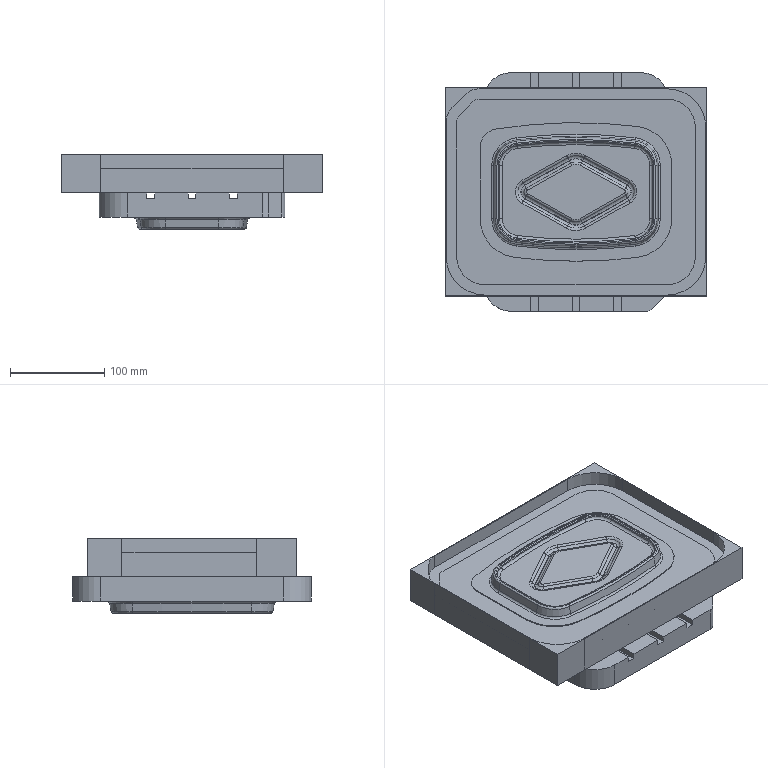NC program | NX | posted with a generic post | part box 278.144 x 254.144 x 79 mm
Lines 4246 to 4920 of 124328:
(CAVITY_MILL_1_COPY , TOOL : D4)
N8490 M6
N8492 G53
N8494 G17 G0 G90 X71.275 Y-37.886 S7000 M3 M8
N8496 G43 Z100.5 H0
N8498 Z37.033
N8500 G94 G1 Z36.033 F4500.
N8502 X72.559 Y-38.883
N8504 G3 X73.682 Y-38.742 R0.8
N8506 G1 X73.795 Y-38.595
N8508 X73.823 Y-38.558
N8510 G3 X74.043 Y-38.269 R17.033
N8512 G2 X76.737 Y-37.786 R2.
N8514 X66.818 Y-46.033 R18.553
N8516 X64.72 Y-46.628 R23.515
N8518 X65.993 Y-44.199 R2.
N8520 G3 X73.309 Y-39.205 R16.805
N8522 G1 X73.341 Y-39.166
N8524 G3 X73.682 Y-38.742 R16.926
N8526 X73.541 Y-37.619 R0.8
N8528 G1 X72.275 Y-36.637
N8530 Z37.033
N8532 G0 Z43.5
N8534 X60.026 Y-40.649
N8536 Z35.13
N8538 G1 Z34.13
N8540 X60.404 Y-42.151
N8542 G3 X61.375 Y-42.731 R0.8
N8544 G1 X61.449 Y-42.712
N8546 G2 X63.94 Y-44.23 R2.
N8548 X63.391 Y-44.336 R16.076
N8550 G1 X62.289 Y-44.523
N8552 G3 X61.928 Y-44.677 R0.84
N8554 G2 X59.759 Y-44.937 R511.246
N8556 X61.301 Y-42.749 R2.
N8558 G1 X61.375 Y-42.731
N8560 G3 X61.956 Y-41.76 R0.8
N8562 G1 X61.577 Y-40.258
N8564 Z35.13
N8566 G0 Z39.033
N8568 X73.119 Y-30.779
N8570 Z35.13
N8572 G1 Z34.13
N8574 X75.709 Y-31.085
N8576 G3 X76.597 Y-30.385 R0.8
N8578 X76.696 Y-29.123 R16.076
N8580 G2 X76.842 Y-28.323 R2.892
N8582 G1 Y-26.204
N8584 G3 X76.042 Y-25.404 R0.8
N8586 G1 X73.448
N8588 Z35.13
N8590 G0 Z41.65
N8592 X-2.129 Y103.007
N8594 Z27.506
N8596 G1 Z26.506
N8598 Y106.722
N8600 G3 X-2.929 Y107.522 R0.8
N8602 G1 X97.072
N8604 G2 X135.922 Y68.672 R38.85
N8606 G1 Y-68.672
N8608 G2 X97.072 Y-107.522 R38.85
N8610 G1 X-97.072
N8612 G2 X-135.922 Y-68.672 R38.85
N8614 G1 Y74.53
N8616 G2 X-130.401 Y87.859 R18.85
N8618 G1 X-116.259 Y102.001
N8620 G2 X-102.93 Y107.522 R18.85
N8622 G1 X-2.929
N8624 Y105.722
N8626 X97.072
N8628 G2 X134.122 Y68.672 R37.05
N8630 G1 Y-68.672
N8632 G2 X97.072 Y-105.722 R37.05
N8634 G1 X-97.072
N8636 G2 X-134.122 Y-68.672 R37.05
N8638 G1 Y74.53
N8640 G2 X-129.128 Y86.586 R17.05
N8642 G1 X-114.986 Y100.728
N8644 G2 X-102.93 Y105.722 R17.05
N8646 G1 X-2.929
N8648 G3 X-2.129 Y106.522 R0.8
N8650 G1 Y103.007
N8652 Z27.506
N8654 G0 Z29.756
N8656 Y103.006 Z27.256
N8658 G1 Z26.256
N8660 Y106.722
N8662 G3 X-2.929 Y107.522 R0.8
N8664 G1 X97.072
N8666 G2 X135.922 Y68.672 R38.85
N8668 G1 Y-68.672
N8670 G2 X97.072 Y-107.522 R38.85
N8672 G1 X-97.072
N8674 G2 X-135.922 Y-68.672 R38.85
N8676 G1 Y74.53
N8678 G2 X-130.401 Y87.859 R18.85
N8680 G1 X-116.259 Y102.001
N8682 G2 X-102.93 Y107.522 R18.85
N8684 G1 X-2.929
N8686 Y105.722
N8688 X97.072
N8690 G2 X134.122 Y68.672 R37.05
N8692 G1 Y-68.672
N8694 G2 X97.072 Y-105.722 R37.05
N8696 G1 X-97.072
N8698 G2 X-134.122 Y-68.672 R37.05
N8700 G1 Y74.53
N8702 G2 X-129.128 Y86.586 R17.05
N8704 G1 X-114.986 Y100.728
N8706 G2 X-102.93 Y105.722 R17.05
N8708 G1 X-2.929
N8710 G3 X-2.129 Y106.522 R0.8
N8712 G1 Y103.006
N8714 Z27.256
N8716 G0 Z29.506
N8718 X-26.78 Y107.522
N8720 Z27.256
N8722 G1 X-2.929 Z26.006
N8724 X97.072
N8726 G2 X135.922 Y68.672 R38.85
N8728 G1 Y-68.672
N8730 G2 X97.072 Y-107.522 R38.85
N8732 G1 X-97.072
N8734 G2 X-135.922 Y-68.672 R38.85
N8736 G1 Y74.53
N8738 G2 X-130.401 Y87.859 R18.85
N8740 G1 X-116.259 Y102.001
N8742 G2 X-102.93 Y107.522 R18.85
N8744 G1 X-2.929
N8746 Y105.722
N8748 X97.072
N8750 G2 X134.122 Y68.672 R37.05
N8752 G1 Y-68.672
N8754 G2 X97.072 Y-105.722 R37.05
N8756 G1 X-97.072
N8758 G2 X-134.122 Y-68.672 R37.05
N8760 G1 Y74.53
N8762 G2 X-129.128 Y86.586 R17.05
N8764 G1 X-114.986 Y100.728
N8766 G2 X-102.93 Y105.722 R17.05
N8768 G1 X-2.929
N8770 G3 X-2.129 Y106.522 R0.8
N8772 G1 Y102.782
N8774 Z27.006
N8776 G0 Z29.256
N8778 X-26.78 Y107.522
N8780 Z27.006
N8782 G1 X-2.929 Z25.756
N8784 X97.072
N8786 G2 X135.922 Y68.672 R38.85
N8788 G1 Y-68.672
N8790 G2 X97.072 Y-107.522 R38.85
N8792 G1 X-97.072
N8794 G2 X-135.922 Y-68.672 R38.85
N8796 G1 Y74.53
N8798 G2 X-130.401 Y87.859 R18.85
N8800 G1 X-116.259 Y102.001
N8802 G2 X-102.93 Y107.522 R18.85
N8804 G1 X-2.929
N8806 Y105.722
N8808 X97.072
N8810 G2 X134.122 Y68.672 R37.05
N8812 G1 Y-68.672
N8814 G2 X97.072 Y-105.722 R37.05
N8816 G1 X-97.072
N8818 G2 X-134.122 Y-68.672 R37.05
N8820 G1 Y74.53
N8822 G2 X-129.128 Y86.586 R17.05
N8824 G1 X-114.986 Y100.728
N8826 G2 X-102.93 Y105.722 R17.05
N8828 G1 X-2.929
N8830 G3 X-2.129 Y106.522 R0.8
N8832 G1 Y102.382
N8834 Z26.756
N8836 G0 Z41.65
N8838 X11.778 Y34.008
N8840 Z35.13
N8842 G1 X32.543 Y22.591 Z33.889
N8844 X55.835 Y9.784
N8846 G2 X55.951 Y-8.882 R10.688
N8848 G1 X8.639 Y-35.664
N8850 G2 X-8.677 Y-35.713 R17.663
N8852 G1 X-55.899 Y-9.33
N8854 G2 X-55.888 Y9.336 R10.688
N8856 G1 X-8.535 Y35.722
N8858 G2 X8.573 Y35.771 R17.663
N8860 G1 X32.543 Y22.591
N8862 X31.194 Y20.137
N8864 X54.486 Y7.33
N8866 G2 X54.572 Y-6.446 R7.888
N8868 G1 X7.26 Y-33.227
N8870 G2 X-7.312 Y-33.268 R14.863
N8872 G1 X-54.533 Y-6.886
N8874 G2 X-54.525 Y6.89 R7.888
N8876 G1 X-7.172 Y33.276
N8878 G2 X7.224 Y33.317 R14.863
N8880 G1 X31.194 Y20.137
N8882 X30.327 Y18.56
N8884 X53.619 Y5.753
N8886 G2 X53.685 Y-4.879 R6.088
N8888 G1 X6.373 Y-31.661
N8890 G2 X-6.434 Y-31.697 R13.063
N8892 G1 X-53.655 Y-5.315
N8894 G2 X-53.649 Y5.318 R6.088
N8896 G1 X-6.296 Y31.704
N8898 G2 X6.356 Y31.74 R13.063
N8900 G1 X30.327 Y18.56
N8902 G3 X31.413 Y18.875 R0.8
N8904 G1 Z34.889
N8906 G0 Z37.13
N8908 X7.26 Y-33.227
N8910 Z34.889
N8912 G1 Z33.889
N8914 X5.963 Y-30.937
N8916 G2 X-6.028 Y-30.971 R12.232
N8918 G1 X-53.25 Y-4.589
N8920 G2 X-53.245 Y4.592 R5.256
N8922 G1 X-5.892 Y30.978
N8924 G2 X5.956 Y31.011 R12.232
N8926 G1 X53.219 Y5.024
N8928 G2 X53.275 Y-4.156 R5.256
N8930 G1 X5.963 Y-30.937
N8932 G3 X5.661 Y-32.028 R0.8
N8934 G1 Z34.889
N8936 G0 Z37.13
N8938 X11.211 Y33.779
N8940 Z34.889
N8942 G1 X31.975 Y22.362 Z33.647
N8944 X55.607 Y9.368
N8946 G2 X55.717 Y-8.47 R10.213
N8948 G1 X8.405 Y-35.251
N8950 G2 X-8.446 Y-35.298 R17.189
N8952 G1 X-55.667 Y-8.916
N8954 G2 X-55.657 Y8.922 R10.213
N8956 G1 X-8.304 Y35.308
N8958 G2 X8.344 Y35.355 R17.189
N8960 G1 X31.975 Y22.362
N8962 X30.626 Y19.908
N8964 X54.258 Y6.915
N8966 G2 X54.338 Y-6.033 R7.413
N8968 G1 X7.026 Y-32.815
N8970 G2 X-7.08 Y-32.854 R14.389
N8972 G1 X-54.302 Y-6.472
N8974 G2 X-54.294 Y6.476 R7.413
N8976 G1 X-6.941 Y32.862
N8978 G2 X6.995 Y32.901 R14.389
N8980 G1 X30.626 Y19.908
N8982 X29.816 Y18.434
N8984 X53.447 Y5.44
N8986 G2 X53.509 Y-4.569 R5.731
N8988 G1 X6.197 Y-31.35
N8990 G2 X-6.26 Y-31.385 R12.706
N8992 G1 X-53.481 Y-5.003
N8994 G2 X-53.475 Y5.006 R5.731
N8996 G1 X-6.122 Y31.392
N8998 G2 X6.184 Y31.427 R12.706
N9000 G1 X29.816 Y18.434
N9002 G3 X30.902 Y18.749 R0.8
N9004 G1 Z34.647
N9006 G0 Z36.889
N9008 X11.047 Y33.481
N9010 Z34.647
N9012 G1 X31.812 Y22.064 Z33.405
N9014 X55.443 Y9.07
N9016 G2 X55.55 Y-8.174 R9.873
N9018 G1 X8.238 Y-34.955
N9020 G2 X-8.28 Y-35.002 R16.849
N9022 G1 X-55.502 Y-8.619
N9024 G2 X-55.492 Y8.625 R9.873
N9026 G1 X-8.139 Y35.011
N9028 G2 X8.18 Y35.057 R16.849
N9030 G1 X31.812 Y22.064
N9032 X30.463 Y19.61
N9034 X54.094 Y6.617
N9036 G2 X54.17 Y-5.737 R7.073
N9038 G1 X6.858 Y-32.519
N9040 G2 X-6.914 Y-32.557 R14.049
N9042 G1 X-54.136 Y-6.175
N9044 G2 X-54.129 Y6.179 R7.073
N9046 G1 X-6.776 Y32.565
N9048 G2 X6.831 Y32.603 R14.049
N9050 G1 X30.463 Y19.61
N9052 X29.98 Y18.731
N9054 X53.611 Y5.738
N9056 G2 X53.677 Y-4.864 R6.071
N9058 G1 X6.364 Y-31.646
N9060 G2 X-6.425 Y-31.682 R13.046
N9062 G1 X-53.647 Y-5.3
N9064 G2 X-53.641 Y5.303 R6.071
N9066 G1 X-6.288 Y31.689
N9068 G2 X6.348 Y31.725 R13.046
N9070 G1 X29.98 Y18.731
N9072 G3 X31.066 Y19.047 R0.8
N9074 G1 Z34.405
N9076 G0 Z36.647
N9078 X11.417 Y32.974
N9080 Z34.405
N9082 G1 X32.182 Y21.557 Z33.163
N9084 X55.315 Y8.837
N9086 G2 X55.419 Y-7.943 R9.608
N9088 G1 X8.107 Y-34.724
N9090 G2 X-8.15 Y-34.77 R16.583
N9092 G1 X-55.372 Y-8.387
N9094 G2 X-55.363 Y8.393 R9.608
N9096 G1 X-8.01 Y34.779
N9098 G2 X8.052 Y34.824 R16.583
N9100 G1 X32.182 Y21.557
N9102 X31.315 Y19.979
N9104 X54.448 Y7.26
N9106 G2 X54.532 Y-6.376 R7.808
N9108 G1 X7.22 Y-33.158
N9110 G2 X-7.273 Y-33.198 R14.783
N9112 G1 X-54.494 Y-6.816
N9114 G2 X-54.486 Y6.82 R7.808
N9116 G1 X-7.133 Y33.206
N9118 G2 X7.185 Y33.247 R14.783
N9120 G1 X31.315 Y19.979
N9122 G3 X32.401 Y20.295 R0.8
N9124 G1 Z34.163
N9126 G0 Z36.405
N9128 X8.107 Y-34.724
N9130 Z34.163
N9132 G1 Z33.163
N9134 X6.495 Y-31.877
N9136 G2 X-6.555 Y-31.914 R13.312
N9138 G1 X-53.777 Y-5.532
N9140 G2 X-53.77 Y5.535 R6.336
N9142 G1 X-6.417 Y31.921
N9144 G2 X6.476 Y31.958 R13.312
N9146 G1 X53.739 Y5.971
N9148 G2 X53.807 Y-5.096 R6.336
N9150 G1 X6.495 Y-31.877
N9152 G3 X6.193 Y-32.968 R0.8
N9154 G1 Z34.163
N9156 G0 Z36.405
N9158 X11.314 Y32.786
N9160 Z34.163
N9162 G1 X32.078 Y21.368 Z32.921
N9164 X55.211 Y8.649
N9166 G2 X55.313 Y-7.755 R9.393
N9168 G1 X8.001 Y-34.537
N9170 G2 X-8.046 Y-34.582 R16.368
N9172 G1 X-55.267 Y-8.2
N9174 G2 X-55.258 Y8.205 R9.393
N9176 G1 X-7.905 Y34.591
N9178 G2 X7.949 Y34.636 R16.368
N9180 G1 X32.078 Y21.368
N9182 X31.211 Y19.791
N9184 X54.344 Y7.072
N9186 G2 X54.426 Y-6.189 R7.593
N9188 G1 X7.114 Y-32.971
N9190 G2 X-7.168 Y-33.011 R14.568
N9192 G1 X-54.389 Y-6.628
N9194 G2 X-54.382 Y6.632 R7.593
N9196 G1 X-7.029 Y33.019
N9198 G2 X7.081 Y33.058 R14.568
N9200 G1 X31.211 Y19.791
N9202 G3 X32.298 Y20.107 R0.8
N9204 G1 Z33.921
N9206 G0 Z37.13
N9208 X8.001 Y-34.537
N9210 Z33.921
N9212 G1 Z32.921
N9214 X6.601 Y-32.065
N9216 G2 X-6.66 Y-32.102 R13.527
N9218 G1 X-53.881 Y-5.719
N9220 G2 X-53.875 Y5.723 R6.551
N9222 G1 X-6.522 Y32.109
N9224 G2 X6.58 Y32.146 R13.527
N9226 G1 X53.843 Y6.159
N9228 G2 X53.913 Y-5.283 R6.551
N9230 G1 X6.601 Y-32.065
N9232 G3 X6.299 Y-33.155 R0.8
N9234 G1 Z33.921
N9236 G0 Z37.13
N9238 X11.229 Y32.631
N9240 Z33.921
N9242 G1 X31.993 Y21.214 Z32.679
N9244 X55.126 Y8.494
N9246 G2 X55.226 Y-7.602 R9.216
N9248 G1 X7.914 Y-34.383
N9250 G2 X-7.96 Y-34.428 R16.192
N9252 G1 X-55.181 Y-8.046
N9254 G2 X-55.172 Y8.051 R9.216
N9256 G1 X-7.819 Y34.437
N9258 G2 X7.864 Y34.481 R16.192
N9260 G1 X31.993 Y21.214
N9262 X31.126 Y19.636
N9264 X54.259 Y6.917
N9266 G2 X54.339 Y-6.035 R7.416
N9268 G1 X7.027 Y-32.817
N9270 G2 X-7.082 Y-32.856 R14.392
N9272 G1 X-54.303 Y-6.474
N9274 G2 X-54.296 Y6.478 R7.416
N9276 G1 X-6.943 Y32.864
N9278 G2 X6.996 Y32.904 R14.392
N9280 G1 X31.126 Y19.636
N9282 G3 X32.213 Y19.952 R0.8
N9284 G1 Z33.679
N9286 G0 Z37.13
N9288 X7.914 Y-34.383
N9290 Z33.679
N9292 G1 Z32.679
N9294 X6.688 Y-32.218
N9296 G2 X-6.746 Y-32.256 R13.703
N9298 G1 X-53.967 Y-5.873
N9300 G2 X-53.961 Y5.877 R6.728
N9302 G1 X-6.608 Y32.263
N9304 G2 X6.665 Y32.301 R13.703
N9306 G1 X53.928 Y6.314
N9308 G2 X54. Y-5.436 R6.728
N9310 G1 X6.688 Y-32.218
N9312 G3 X6.386 Y-33.308 R0.8
N9314 G1 Z33.679
N9316 G0 Z37.13
N9318 X11.146 Y32.48
N9320 Z33.679
N9322 G1 X31.91 Y21.063 Z32.437
N9324 X55.043 Y8.343
N9326 G2 X55.141 Y-7.452 R9.044
N9328 G1 X7.829 Y-34.234
N9330 G2 X-7.875 Y-34.277 R16.019
N9332 G1 X-55.097 Y-7.895
N9334 G2 X-55.088 Y7.9 R9.044
N9336 G1 X-7.735 Y34.286
N9338 G2 X7.781 Y34.33 R16.019
N9340 G1 X31.91 Y21.063
N9342 X30.878 Y19.184
N9344 X54.011 Y6.465
N9346 G2 X54.085 Y-5.586 R6.9
N9348 G1 X6.773 Y-32.368
N9350 G2 X-6.83 Y-32.406 R13.876
N9352 G1 X-54.052 Y-6.024
N9354 G2 X-54.045 Y6.028 R6.9
N9356 G1 X-6.692 Y32.414
N9358 G2 X6.748 Y32.452 R13.876
N9360 G1 X30.878 Y19.184
N9362 G3 X31.964 Y19.5 R0.8
N9364 G1 Z33.437
N9366 G0 Z35.679
N9368 X11.047 Y32.301
N9370 Z33.437
N9372 G1 X31.812 Y20.884 Z32.195
N9374 X54.945 Y8.165
N9376 G2 X55.041 Y-7.274 R8.84
N9378 G1 X7.728 Y-34.056
N9380 G2 X-7.776 Y-34.099 R15.815
N9382 G1 X-54.997 Y-7.717
N9384 G2 X-54.989 Y7.722 R8.84
N9386 G1 X-7.636 Y34.108
N9388 G2 X7.682 Y34.151 R15.815
N9390 G1 X31.812 Y20.884
N9392 X30.976 Y19.363
N9394 X54.109 Y6.644
N9396 G2 X54.186 Y-5.764 R7.104
N9398 G1 X6.874 Y-32.546
N9400 G2 X-6.93 Y-32.584 R14.08
N9402 G1 X-54.151 Y-6.202
N9404 G2 X-54.144 Y6.206 R7.104
N9406 G1 X-6.791 Y32.592
N9408 G2 X6.846 Y32.631 R14.08
N9410 G1 X30.976 Y19.363
N9412 G3 X32.062 Y19.679 R0.8
N9414 G1 Z33.195
N9416 G0 Z35.437
N9418 X10.431 Y32.362
N9420 Z33.195
N9422 G1 X31.196 Y20.944 Z31.953
N9424 X54.828 Y7.951
N9426 G2 X54.921 Y-7.062 R8.596
N9428 G1 X7.608 Y-33.844
N9430 G2 X-7.657 Y-33.887 R15.572
N9432 G1 X-54.879 Y-7.504
N9434 G2 X-54.87 Y7.509 R8.596
N9436 G1 X-7.517 Y33.895
N9438 G2 X7.565 Y33.938 R15.572
N9440 G1 X31.196 Y20.944
N9442 X30.595 Y19.851
N9444 X54.226 Y6.857
N9446 G2 X54.306 Y-5.976 R7.348
N9448 G1 X6.994 Y-32.758
N9450 G2 X-7.048 Y-32.797 R14.323
N9452 G1 X-54.27 Y-6.415
N9454 G2 X-54.263 Y6.419 R7.348
N9456 G1 X-6.91 Y32.805
N9458 G2 X6.964 Y32.844 R14.323
N9460 G1 X30.595 Y19.851
N9462 G3 X31.681 Y20.166 R0.8
N9464 G1 Z32.953
N9466 G0 Z35.195
N9468 X10.289 Y32.102
N9470 Z32.953
N9472 G1 X31.053 Y20.685 Z31.712
N9474 X54.685 Y7.691
N9476 G2 X54.775 Y-6.804 R8.3
N9478 G1 X7.462 Y-33.586
N9480 G2 X-7.513 Y-33.628 R15.275
N9482 G1 X-54.734 Y-7.246
N9484 G2 X-54.726 Y7.25 R8.3
N9486 G1 X-7.373 Y33.636
N9488 G2 X7.422 Y33.678 R15.275
N9490 G1 X31.053 Y20.685
N9492 X30.738 Y20.11
N9494 X54.369 Y7.117
N9496 G2 X54.452 Y-6.234 R7.644
N9498 G1 X7.14 Y-33.016
N9500 G2 X-7.193 Y-33.056 R14.62
N9502 G1 X-54.414 Y-6.673
N9504 G2 X-54.407 Y6.678 R7.644
N9506 G1 X-7.054 Y33.064
N9508 G2 X7.106 Y33.104 R14.62
N9510 G1 X30.738 Y20.11
N9512 G3 X31.281 Y20.268 R0.4
N9514 G1 Z32.712
N9516 G0 Z41.65
N9518 X-108.649 Y8.666
N9520 Z27.506
N9522 G1 Z26.506
N9524 X-107.049
N9526 G3 X-106.249 Y9.466 R0.8
N9528 G1 Y47.133
N9530 G2 X-85.957 Y70.972 R24.149
N9532 G1 X-85.955
N9534 G2 X65.889 Y73.819 R540.653
N9536 X106.249 Y28.201 R45.961
N9538 G1 Y-28.201
N9540 G2 X65.889 Y-73.819 R45.961
N9542 X-65.889 Y-73.819 R540.653
N9544 X-106.249 Y-28.201 R45.961
N9546 G1 Y9.466
N9548 X-104.222
N9550 Y47.133
N9552 G2 X-85.616 Y68.974 R22.122
N9554 X65.642 Y71.807 R538.627
N9556 X104.222 Y28.201 R43.934
N9558 G1 Y-28.201
N9560 G2 X65.642 Y-71.807 R43.934
N9562 X-65.642 Y-71.807 R538.627
N9564 X-104.222 Y-28.201 R43.934
N9566 G1 Y9.466
N9568 G3 X-105.022 Y10.266 R0.8
N9570 G1 X-108.649
N9572 Z27.506
N9574 G0 Z29.756
N9576 X-108.726 Y8.666
N9578 Z27.256
N9580 G1 Z26.256
N9582 X-107.126
N9584 G3 X-106.326 Y9.466 R0.8
N9586 G1 Y46.996
N9588 X-106.325 Y47.066
N9590 Y47.133
N9592 G2 X-85.952 Y71.051 R24.226
N9594 X65.856 Y73.9 R540.73
N9596 G1 X65.859
N9598 X65.863 Y73.899
N9600 G2 X106.325 Y28.421 R46.037
N9602 G1 X106.324 Y28.3
N9604 G3 X106.324 Y28.093 R3.884
N9606 G1 X106.326 Y27.981
N9608 Y-27.981
N9610 X106.324 Y-28.092
N9612 G3 X106.324 Y-28.3 R3.884
N9614 G1 X106.325 Y-28.421
N9616 G2 X65.904 Y-73.894 R46.037
N9618 X-65.856 Y-73.9 R540.73
N9620 G1 X-65.86
N9622 G2 X-106.325 Y-28.421 R46.037
N9624 G1 X-106.324 Y-28.3
N9626 G3 X-106.324 Y-28.093 R3.885
N9628 G1 X-106.326 Y-27.981
N9630 Y9.466
N9632 X-104.222
N9634 Y47.133
N9636 G2 X-85.616 Y68.974 R22.122
N9638 X65.642 Y71.807 R538.627
N9640 X104.222 Y28.201 R43.934
N9642 G1 Y-28.201
N9644 G2 X65.642 Y-71.807 R43.934
N9646 X-65.642 Y-71.807 R538.627
N9648 X-104.222 Y-28.201 R43.934
N9650 G1 Y9.466
N9652 G3 X-105.022 Y10.266 R0.8
N9654 G1 X-108.726
N9656 Z27.256
N9658 G0 Z29.506
N9660 X-108.958 Y8.666
N9662 Z27.006
N9664 G1 Z26.006
N9666 X-107.358
N9668 G3 X-106.558 Y9.466 R0.8
N9670 G1 Y47.017
N9672 X-106.557 Y47.078
N9674 Y47.133
N9676 G2 X-85.988 Y71.28 R24.457
N9678 G1 X-85.987
N9680 G2 X65.885 Y74.13 R540.962
N9682 G1 X65.883
N9684 X65.888
N9686 G2 X106.558 Y28.163 R46.269
N9688 G1 Y28.16
N9690 Y-28.16
N9692 Y-28.163
N9694 G2 X65.959 Y-74.121 R46.269
N9696 G1 X65.957
N9698 G2 X-65.885 Y-74.13 R540.962
N9700 G1 X-65.887
N9702 X-65.89
N9704 G2 X-106.558 Y-28.163 R46.269
N9706 G1 Y-28.16
N9708 Y9.466
N9710 X-104.222
N9712 Y47.133
N9714 G2 X-85.616 Y68.974 R22.122
N9716 X65.642 Y71.807 R538.627
N9718 X104.222 Y28.201 R43.934
N9720 G1 Y-28.201
N9722 G2 X65.642 Y-71.807 R43.934
N9724 X-65.642 Y-71.807 R538.627
N9726 X-104.222 Y-28.201 R43.934
N9728 G1 Y9.466
N9730 G3 X-105.022 Y10.266 R0.8
N9732 G1 X-108.958
N9734 Z27.006
N9736 G0 Z29.256
N9738 X-109.362 Y8.666
N9740 Z26.756
N9742 G1 Z25.756
N9744 X-107.762
N9746 G3 X-106.962 Y9.466 R0.8
N9748 G1 Y47.133
N9750 G2 X-86.052 Y71.679 R24.862
N9752 X65.976 Y74.527 R541.367
N9754 X106.962 Y28.201 R46.674
N9756 G1 Y-28.201
N9758 G2 X65.957 Y-74.529 R46.674
N9760 G1 X65.954
N9762 G2 X-65.976 Y-74.527 R541.367
N9764 G1 X-65.977 Y-74.526
N9766 G2 X-106.962 Y-28.201 R46.674
N9768 G1 Y9.466
N9770 X-105.162
N9772 Y47.133
N9774 G2 X-85.766 Y69.902 R23.062
N9776 X65.757 Y72.74 R539.567
N9778 X105.162 Y28.201 R44.874
N9780 G1 Y-28.201
N9782 G2 X65.738 Y-72.742 R44.874
N9784 X-65.757 Y-72.74 R539.567
N9786 X-105.162 Y-28.201 R44.874
N9788 G1 Y9.466
N9790 G3 X-105.962 Y10.266 R0.8
N9792 G1 X-109.362
N9794 Z26.756
N9796 G0 Z29.006
N9798 X-86.052 Y71.679
N9800 Z26.756
N9802 G1 Z25.756
N9804 X-85.616 Y68.974
N9806 G2 X65.642 Y71.807 R538.627
N9808 X104.222 Y28.201 R43.934
N9810 G1 Y-28.201
N9812 G2 X65.642 Y-71.807 R43.934
N9814 X-65.642 Y-71.807 R538.627
N9816 X-104.222 Y-28.201 R43.934
N9818 G1 Y47.133
N9820 G2 X-85.616 Y68.974 R22.122
N9822 G3 X-84.954 Y69.891 R0.8
N9824 G1 X-85.644 Y74.175
N9826 Z26.756
N9828 G0 Z100.5
N9830 M9
N9832 M5